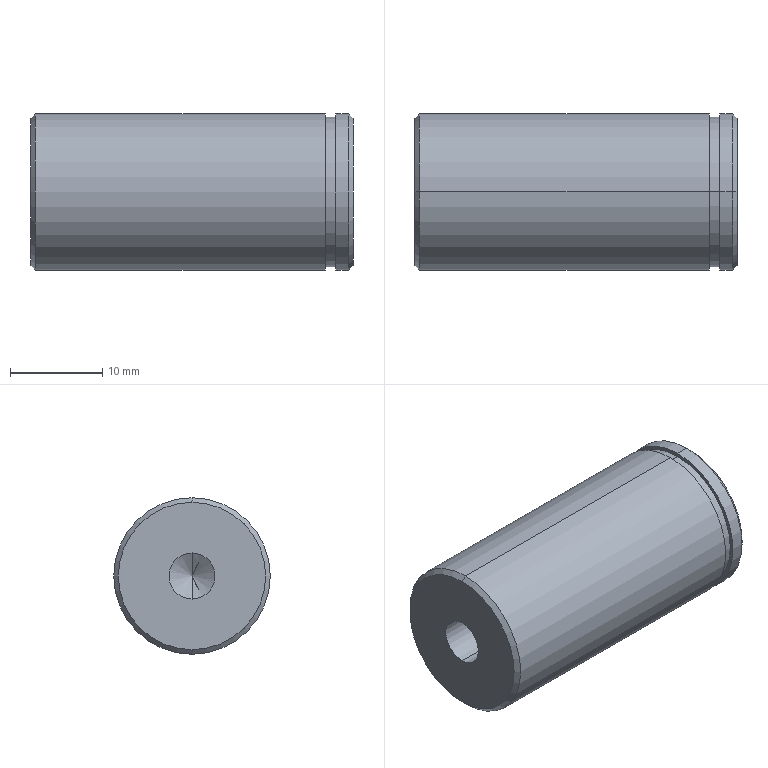Part | SolidWorks | features Chamfer 1, Extrusion 1, HoleWzd 1, RevCut 1 | 1 solid | 18 faces | box 35 x 17 x 17 mm | volume 7604 mm3 | cylinder 8 | cone 6 | plane 4 | commonest cylinder face diameters 17 x4 5 x2 16.2 x2
STEP:
#1=CARTESIAN_POINT('',(34.5,0.,8.5));
#2=VERTEX_POINT('',#1);
#3=CARTESIAN_POINT('',(34.5,0.,-8.5));
#4=VERTEX_POINT('',#3);
#5=CARTESIAN_POINT('',(34.5,0.,0.));
#6=DIRECTION('',(-1.,0.,0.));
#7=DIRECTION('',(0.,0.,-1.));
#8=AXIS2_PLACEMENT_3D('',#5,#6,#7);
#9=CIRCLE('',#8,8.5);
#10=EDGE_CURVE('',#2,#4,#9,.T.);
#11=ORIENTED_EDGE('',*,*,#10,.T.);
#12=CARTESIAN_POINT('',(33.1,0.,-8.5));
#13=VERTEX_POINT('',#12);
#14=CARTESIAN_POINT('',(35.,0.,-8.5));
#15=DIRECTION('',(-1.,0.,0.));
#16=VECTOR('',#15,1000.);
#17=LINE('',#14,#16);
#18=EDGE_CURVE('',#4,#13,#17,.T.);
#19=ORIENTED_EDGE('',*,*,#18,.T.);
#20=CARTESIAN_POINT('',(33.1,0.,8.5));
#21=VERTEX_POINT('',#20);
#22=CARTESIAN_POINT('',(33.1,0.,0.));
#23=DIRECTION('',(-1.,0.,0.));
#24=DIRECTION('',(0.,0.,1.));
#25=AXIS2_PLACEMENT_3D('',#22,#23,#24);
#26=CIRCLE('',#25,8.5);
#27=EDGE_CURVE('',#21,#13,#26,.T.);
#28=ORIENTED_EDGE('',*,*,#27,.F.);
#29=CARTESIAN_POINT('',(35.,0.,8.5));
#30=DIRECTION('',(-1.,0.,0.));
#31=VECTOR('',#30,1000.);
#32=LINE('',#29,#31);
#33=EDGE_CURVE('',#2,#21,#32,.T.);
#34=ORIENTED_EDGE('',*,*,#33,.F.);
#35=EDGE_LOOP('',(#11,#19,#28,#34));
#36=FACE_OUTER_BOUND('',#35,.T.);
#37=CARTESIAN_POINT('',(35.,0.,0.));
#38=DIRECTION('',(-1.,0.,0.));
#39=DIRECTION('',(0.,0.,1.));
#40=AXIS2_PLACEMENT_3D('',#37,#38,#39);
#41=CYLINDRICAL_SURFACE('',#40,8.5);
#42=ADVANCED_FACE('',(#36),#41,.T.);
#43=CARTESIAN_POINT('',(35.,0.,-8.));
#44=VERTEX_POINT('',#43);
#45=CARTESIAN_POINT('',(35.,0.,8.));
#46=VERTEX_POINT('',#45);
#47=CARTESIAN_POINT('',(35.,0.,0.));
#48=DIRECTION('',(1.,0.,0.));
#49=DIRECTION('',(0.,0.,-1.));
#50=AXIS2_PLACEMENT_3D('',#47,#48,#49);
#51=CIRCLE('',#50,8.);
#52=EDGE_CURVE('',#44,#46,#51,.T.);
#53=ORIENTED_EDGE('',*,*,#52,.F.);
#54=CARTESIAN_POINT('',(35.,0.,-8.));
#55=DIRECTION('',(-0.7071,0.,-0.7071));
#56=VECTOR('',#55,1000.);
#57=LINE('',#54,#56);
#58=EDGE_CURVE('',#44,#4,#57,.T.);
#59=ORIENTED_EDGE('',*,*,#58,.T.);
#60=ORIENTED_EDGE('',*,*,#10,.F.);
#61=CARTESIAN_POINT('',(35.,0.,8.));
#62=DIRECTION('',(-0.7071,0.,0.7071));
#63=VECTOR('',#62,1000.);
#64=LINE('',#61,#63);
#65=EDGE_CURVE('',#46,#2,#64,.T.);
#66=ORIENTED_EDGE('',*,*,#65,.F.);
#67=EDGE_LOOP('',(#53,#59,#60,#66));
#68=FACE_OUTER_BOUND('',#67,.T.);
#69=CARTESIAN_POINT('',(35.,0.,0.));
#70=DIRECTION('',(-1.,0.,0.));
#71=DIRECTION('',(0.,0.,1.));
#72=AXIS2_PLACEMENT_3D('',#69,#70,#71);
#73=CONICAL_SURFACE('',#72,8.,0.7854);
#74=ADVANCED_FACE('',(#68),#73,.T.);
#75=CARTESIAN_POINT('',(33.1,0.,8.1));
#76=VERTEX_POINT('',#75);
#77=CARTESIAN_POINT('',(33.1,0.,-8.1));
#78=VERTEX_POINT('',#77);
#79=CARTESIAN_POINT('',(33.1,0.,0.));
#80=DIRECTION('',(-1.,0.,0.));
#81=DIRECTION('',(0.,0.,1.));
#82=AXIS2_PLACEMENT_3D('',#79,#80,#81);
#83=CIRCLE('',#82,8.1);
#84=EDGE_CURVE('',#76,#78,#83,.T.);
#85=ORIENTED_EDGE('',*,*,#84,.T.);
#86=CARTESIAN_POINT('',(32.,0.,-8.1));
#87=VERTEX_POINT('',#86);
#88=CARTESIAN_POINT('',(-5.278,0.,-8.1));
#89=DIRECTION('',(-1.,0.,0.));
#90=VECTOR('',#89,1000.);
#91=LINE('',#88,#90);
#92=EDGE_CURVE('',#78,#87,#91,.T.);
#93=ORIENTED_EDGE('',*,*,#92,.T.);
#94=CARTESIAN_POINT('',(32.,0.,8.1));
#95=VERTEX_POINT('',#94);
#96=CARTESIAN_POINT('',(32.,0.,0.));
#97=DIRECTION('',(-1.,0.,0.));
#98=DIRECTION('',(0.,0.,1.));
#99=AXIS2_PLACEMENT_3D('',#96,#97,#98);
#100=CIRCLE('',#99,8.1);
#101=EDGE_CURVE('',#95,#87,#100,.T.);
#102=ORIENTED_EDGE('',*,*,#101,.F.);
#103=CARTESIAN_POINT('',(-5.278,0.,8.1));
#104=DIRECTION('',(-1.,0.,0.));
#105=VECTOR('',#104,1000.);
#106=LINE('',#103,#105);
#107=EDGE_CURVE('',#76,#95,#106,.T.);
#108=ORIENTED_EDGE('',*,*,#107,.F.);
#109=EDGE_LOOP('',(#85,#93,#102,#108));
#110=FACE_OUTER_BOUND('',#109,.T.);
#111=CARTESIAN_POINT('',(-5.278,0.,0.));
#112=DIRECTION('',(-1.,0.,0.));
#113=DIRECTION('',(0.,0.,1.));
#114=AXIS2_PLACEMENT_3D('',#111,#112,#113);
#115=CYLINDRICAL_SURFACE('',#114,8.1);
#116=ADVANCED_FACE('',(#110),#115,.T.);
#117=CARTESIAN_POINT('',(0.,0.,8.));
#118=VERTEX_POINT('',#117);
#119=CARTESIAN_POINT('',(0.,0.,-8.));
#120=VERTEX_POINT('',#119);
#121=CARTESIAN_POINT('',(0.,0.,0.));
#122=DIRECTION('',(-1.,0.,0.));
#123=DIRECTION('',(0.,0.,-1.));
#124=AXIS2_PLACEMENT_3D('',#121,#122,#123);
#125=CIRCLE('',#124,8.);
#126=EDGE_CURVE('',#118,#120,#125,.T.);
#127=ORIENTED_EDGE('',*,*,#126,.F.);
#128=CARTESIAN_POINT('',(0.5,0.,8.5));
#129=VERTEX_POINT('',#128);
#130=CARTESIAN_POINT('',(0.5,0.,8.5));
#131=DIRECTION('',(0.7071,0.,0.7071));
#132=VECTOR('',#131,1000.);
#133=LINE('',#130,#132);
#134=EDGE_CURVE('',#118,#129,#133,.T.);
#135=ORIENTED_EDGE('',*,*,#134,.T.);
#136=CARTESIAN_POINT('',(0.5,0.,-8.5));
#137=VERTEX_POINT('',#136);
#138=CARTESIAN_POINT('',(0.5,0.,0.));
#139=DIRECTION('',(1.,0.,0.));
#140=DIRECTION('',(0.,0.,-1.));
#141=AXIS2_PLACEMENT_3D('',#138,#139,#140);
#142=CIRCLE('',#141,8.5);
#143=EDGE_CURVE('',#137,#129,#142,.T.);
#144=ORIENTED_EDGE('',*,*,#143,.F.);
#145=CARTESIAN_POINT('',(0.5,0.,-8.5));
#146=DIRECTION('',(0.7071,0.,-0.7071));
#147=VECTOR('',#146,1000.);
#148=LINE('',#145,#147);
#149=EDGE_CURVE('',#120,#137,#148,.T.);
#150=ORIENTED_EDGE('',*,*,#149,.F.);
#151=EDGE_LOOP('',(#127,#135,#144,#150));
#152=FACE_OUTER_BOUND('',#151,.T.);
#153=CARTESIAN_POINT('',(0.5,0.,0.));
#154=DIRECTION('',(1.,0.,0.));
#155=DIRECTION('',(0.,0.,-1.));
#156=AXIS2_PLACEMENT_3D('',#153,#154,#155);
#157=CONICAL_SURFACE('',#156,8.5,0.7854);
#158=ADVANCED_FACE('',(#152),#157,.T.);
#159=CARTESIAN_POINT('',(15.,0.,-2.5));
#160=VERTEX_POINT('',#159);
#161=CARTESIAN_POINT('',(15.,0.,2.5));
#162=VERTEX_POINT('',#161);
#163=CARTESIAN_POINT('',(15.,0.,0.));
#164=DIRECTION('',(-1.,0.,0.));
#165=DIRECTION('',(0.,0.,1.));
#166=AXIS2_PLACEMENT_3D('',#163,#164,#165);
#167=CIRCLE('',#166,2.5);
#168=EDGE_CURVE('',#160,#162,#167,.T.);
#169=ORIENTED_EDGE('',*,*,#168,.F.);
#170=CARTESIAN_POINT('',(0.,0.,-2.5));
#171=VERTEX_POINT('',#170);
#172=CARTESIAN_POINT('',(0.,0.,-2.5));
#173=DIRECTION('',(-1.,0.,0.));
#174=VECTOR('',#173,1000.);
#175=LINE('',#172,#174);
#176=EDGE_CURVE('',#160,#171,#175,.T.);
#177=ORIENTED_EDGE('',*,*,#176,.T.);
#178=CARTESIAN_POINT('',(0.,0.,2.5));
#179=VERTEX_POINT('',#178);
#180=CARTESIAN_POINT('',(0.,0.,0.));
#181=DIRECTION('',(-1.,0.,0.));
#182=DIRECTION('',(0.,0.,1.));
#183=AXIS2_PLACEMENT_3D('',#180,#181,#182);
#184=CIRCLE('',#183,2.5);
#185=EDGE_CURVE('',#171,#179,#184,.T.);
#186=ORIENTED_EDGE('',*,*,#185,.T.);
#187=CARTESIAN_POINT('',(0.,0.,2.5));
#188=DIRECTION('',(-1.,0.,0.));
#189=VECTOR('',#188,1000.);
#190=LINE('',#187,#189);
#191=EDGE_CURVE('',#162,#179,#190,.T.);
#192=ORIENTED_EDGE('',*,*,#191,.F.);
#193=EDGE_LOOP('',(#169,#177,#186,#192));
#194=FACE_OUTER_BOUND('',#193,.T.);
#195=CARTESIAN_POINT('',(0.,0.,0.));
#196=DIRECTION('',(-1.,0.,0.));
#197=DIRECTION('',(0.,0.,1.));
#198=AXIS2_PLACEMENT_3D('',#195,#196,#197);
#199=CYLINDRICAL_SURFACE('',#198,2.5);
#200=ADVANCED_FACE('',(#194),#199,.F.);
#201=CARTESIAN_POINT('',(16.502,0.,0.));
#202=VERTEX_POINT('',#201);
#203=CARTESIAN_POINT('',(15.,0.,2.5));
#204=DIRECTION('',(-0.515,0.,0.8572));
#205=VECTOR('',#204,1000.);
#206=LINE('',#203,#205);
#207=EDGE_CURVE('',#202,#162,#206,.T.);
#208=ORIENTED_EDGE('',*,*,#207,.F.);
#209=CARTESIAN_POINT('',(15.,0.,-2.5));
#210=DIRECTION('',(-0.515,0.,-0.8572));
#211=VECTOR('',#210,1000.);
#212=LINE('',#209,#211);
#213=EDGE_CURVE('',#202,#160,#212,.T.);
#214=ORIENTED_EDGE('',*,*,#213,.T.);
#215=ORIENTED_EDGE('',*,*,#168,.T.);
#216=EDGE_LOOP('',(#208,#214,#215));
#217=FACE_OUTER_BOUND('',#216,.T.);
#218=CARTESIAN_POINT('',(15.,0.,0.));
#219=DIRECTION('',(-1.,0.,0.));
#220=DIRECTION('',(0.,0.,1.));
#221=AXIS2_PLACEMENT_3D('',#218,#219,#220);
#222=CONICAL_SURFACE('',#221,2.5,1.03);
#223=ADVANCED_FACE('',(#217),#222,.F.);
#224=CARTESIAN_POINT('',(32.,0.,-8.5));
#225=VERTEX_POINT('',#224);
#226=CARTESIAN_POINT('',(32.,0.,8.5));
#227=VERTEX_POINT('',#226);
#228=CARTESIAN_POINT('',(32.,0.,0.));
#229=DIRECTION('',(1.,0.,0.));
#230=DIRECTION('',(0.,0.,-1.));
#231=AXIS2_PLACEMENT_3D('',#228,#229,#230);
#232=CIRCLE('',#231,8.5);
#233=EDGE_CURVE('',#225,#227,#232,.T.);
#234=ORIENTED_EDGE('',*,*,#233,.F.);
#235=CARTESIAN_POINT('',(35.,0.,-8.5));
#236=DIRECTION('',(-1.,0.,0.));
#237=VECTOR('',#236,1000.);
#238=LINE('',#235,#237);
#239=EDGE_CURVE('',#225,#137,#238,.T.);
#240=ORIENTED_EDGE('',*,*,#239,.T.);
#241=ORIENTED_EDGE('',*,*,#143,.T.);
#242=CARTESIAN_POINT('',(35.,0.,8.5));
#243=DIRECTION('',(-1.,0.,0.));
#244=VECTOR('',#243,1000.);
#245=LINE('',#242,#244);
#246=EDGE_CURVE('',#227,#129,#245,.T.);
#247=ORIENTED_EDGE('',*,*,#246,.F.);
#248=EDGE_LOOP('',(#234,#240,#241,#247));
#249=FACE_OUTER_BOUND('',#248,.T.);
#250=CARTESIAN_POINT('',(35.,0.,0.));
#251=DIRECTION('',(-1.,0.,0.));
#252=DIRECTION('',(0.,0.,1.));
#253=AXIS2_PLACEMENT_3D('',#250,#251,#252);
#254=CYLINDRICAL_SURFACE('',#253,8.5);
#255=ADVANCED_FACE('',(#249),#254,.T.);
#256=ORIENTED_EDGE('',*,*,#239,.F.);
#257=CARTESIAN_POINT('',(32.,0.,0.));
#258=DIRECTION('',(1.,0.,0.));
#259=DIRECTION('',(0.,0.,-1.));
#260=AXIS2_PLACEMENT_3D('',#257,#258,#259);
#261=CIRCLE('',#260,8.5);
#262=EDGE_CURVE('',#227,#225,#261,.T.);
#263=ORIENTED_EDGE('',*,*,#262,.F.);
#264=ORIENTED_EDGE('',*,*,#246,.T.);
#265=CARTESIAN_POINT('',(0.5,0.,0.));
#266=DIRECTION('',(1.,0.,0.));
#267=DIRECTION('',(0.,0.,-1.));
#268=AXIS2_PLACEMENT_3D('',#265,#266,#267);
#269=CIRCLE('',#268,8.5);
#270=EDGE_CURVE('',#129,#137,#269,.T.);
#271=ORIENTED_EDGE('',*,*,#270,.T.);
#272=EDGE_LOOP('',(#256,#263,#264,#271));
#273=FACE_OUTER_BOUND('',#272,.T.);
#274=CARTESIAN_POINT('',(35.,0.,0.));
#275=DIRECTION('',(-1.,0.,0.));
#276=DIRECTION('',(0.,0.,1.));
#277=AXIS2_PLACEMENT_3D('',#274,#275,#276);
#278=CYLINDRICAL_SURFACE('',#277,8.5);
#279=ADVANCED_FACE('',(#273),#278,.T.);
#280=CARTESIAN_POINT('',(0.,0.,0.));
#281=DIRECTION('',(-1.,0.,0.));
#282=DIRECTION('',(0.,0.,-1.));
#283=AXIS2_PLACEMENT_3D('',#280,#281,#282);
#284=CIRCLE('',#283,8.);
#285=EDGE_CURVE('',#120,#118,#284,.T.);
#286=ORIENTED_EDGE('',*,*,#285,.T.);
#287=ORIENTED_EDGE('',*,*,#126,.T.);
#288=EDGE_LOOP('',(#286,#287));
#289=FACE_OUTER_BOUND('',#288,.T.);
#290=CARTESIAN_POINT('',(0.,0.,0.));
#291=DIRECTION('',(-1.,0.,0.));
#292=DIRECTION('',(0.,0.,1.));
#293=AXIS2_PLACEMENT_3D('',#290,#291,#292);
#294=CIRCLE('',#293,2.5);
#295=EDGE_CURVE('',#179,#171,#294,.T.);
#296=ORIENTED_EDGE('',*,*,#295,.F.);
#297=ORIENTED_EDGE('',*,*,#185,.F.);
#298=EDGE_LOOP('',(#296,#297));
#299=FACE_BOUND('',#298,.T.);
#300=CARTESIAN_POINT('',(0.,0.,0.));
#301=DIRECTION('',(1.,0.,0.));
#302=DIRECTION('',(0.,0.,-1.));
#303=AXIS2_PLACEMENT_3D('',#300,#301,#302);
#304=PLANE('',#303);
#305=ADVANCED_FACE('',(#289,#299),#304,.F.);
#306=ORIENTED_EDGE('',*,*,#213,.F.);
#307=ORIENTED_EDGE('',*,*,#207,.T.);
#308=CARTESIAN_POINT('',(15.,0.,0.));
#309=DIRECTION('',(-1.,0.,0.));
#310=DIRECTION('',(0.,0.,1.));
#311=AXIS2_PLACEMENT_3D('',#308,#309,#310);
#312=CIRCLE('',#311,2.5);
#313=EDGE_CURVE('',#162,#160,#312,.T.);
#314=ORIENTED_EDGE('',*,*,#313,.T.);
#315=EDGE_LOOP('',(#306,#307,#314));
#316=FACE_OUTER_BOUND('',#315,.T.);
#317=CARTESIAN_POINT('',(15.,0.,0.));
#318=DIRECTION('',(-1.,0.,0.));
#319=DIRECTION('',(0.,0.,1.));
#320=AXIS2_PLACEMENT_3D('',#317,#318,#319);
#321=CONICAL_SURFACE('',#320,2.5,1.03);
#322=ADVANCED_FACE('',(#316),#321,.F.);
#323=ORIENTED_EDGE('',*,*,#176,.F.);
#324=ORIENTED_EDGE('',*,*,#313,.F.);
#325=ORIENTED_EDGE('',*,*,#191,.T.);
#326=ORIENTED_EDGE('',*,*,#295,.T.);
#327=EDGE_LOOP('',(#323,#324,#325,#326));
#328=FACE_OUTER_BOUND('',#327,.T.);
#329=CARTESIAN_POINT('',(0.,0.,0.));
#330=DIRECTION('',(-1.,0.,0.));
#331=DIRECTION('',(0.,0.,1.));
#332=AXIS2_PLACEMENT_3D('',#329,#330,#331);
#333=CYLINDRICAL_SURFACE('',#332,2.5);
#334=ADVANCED_FACE('',(#328),#333,.F.);
#335=ORIENTED_EDGE('',*,*,#134,.F.);
#336=ORIENTED_EDGE('',*,*,#285,.F.);
#337=ORIENTED_EDGE('',*,*,#149,.T.);
#338=ORIENTED_EDGE('',*,*,#270,.F.);
#339=EDGE_LOOP('',(#335,#336,#337,#338));
#340=FACE_OUTER_BOUND('',#339,.T.);
#341=CARTESIAN_POINT('',(0.5,0.,0.));
#342=DIRECTION('',(1.,0.,0.));
#343=DIRECTION('',(0.,0.,-1.));
#344=AXIS2_PLACEMENT_3D('',#341,#342,#343);
#345=CONICAL_SURFACE('',#344,8.5,0.7854);
#346=ADVANCED_FACE('',(#340),#345,.T.);
#347=ORIENTED_EDGE('',*,*,#101,.T.);
#348=CARTESIAN_POINT('',(32.,0.,0.));
#349=DIRECTION('',(-1.,0.,0.));
#350=DIRECTION('',(0.,0.,1.));
#351=AXIS2_PLACEMENT_3D('',#348,#349,#350);
#352=CIRCLE('',#351,8.1);
#353=EDGE_CURVE('',#87,#95,#352,.T.);
#354=ORIENTED_EDGE('',*,*,#353,.T.);
#355=EDGE_LOOP('',(#347,#354));
#356=FACE_BOUND('',#355,.T.);
#357=ORIENTED_EDGE('',*,*,#262,.T.);
#358=ORIENTED_EDGE('',*,*,#233,.T.);
#359=EDGE_LOOP('',(#357,#358));
#360=FACE_OUTER_BOUND('',#359,.T.);
#361=CARTESIAN_POINT('',(32.,0.,-10.865));
#362=DIRECTION('',(1.,0.,0.));
#363=DIRECTION('',(0.,0.,-1.));
#364=AXIS2_PLACEMENT_3D('',#361,#362,#363);
#365=PLANE('',#364);
#366=ADVANCED_FACE('',(#356,#360),#365,.T.);
#367=ORIENTED_EDGE('',*,*,#84,.F.);
#368=CARTESIAN_POINT('',(33.1,0.,0.));
#369=DIRECTION('',(-1.,0.,0.));
#370=DIRECTION('',(0.,0.,1.));
#371=AXIS2_PLACEMENT_3D('',#368,#369,#370);
#372=CIRCLE('',#371,8.1);
#373=EDGE_CURVE('',#78,#76,#372,.T.);
#374=ORIENTED_EDGE('',*,*,#373,.F.);
#375=EDGE_LOOP('',(#367,#374));
#376=FACE_BOUND('',#375,.T.);
#377=ORIENTED_EDGE('',*,*,#27,.T.);
#378=CARTESIAN_POINT('',(33.1,0.,0.));
#379=DIRECTION('',(-1.,0.,0.));
#380=DIRECTION('',(0.,0.,1.));
#381=AXIS2_PLACEMENT_3D('',#378,#379,#380);
#382=CIRCLE('',#381,8.5);
#383=EDGE_CURVE('',#13,#21,#382,.T.);
#384=ORIENTED_EDGE('',*,*,#383,.T.);
#385=EDGE_LOOP('',(#377,#384));
#386=FACE_OUTER_BOUND('',#385,.T.);
#387=CARTESIAN_POINT('',(33.1,0.,-10.865));
#388=DIRECTION('',(-1.,0.,0.));
#389=DIRECTION('',(0.,0.,1.));
#390=AXIS2_PLACEMENT_3D('',#387,#388,#389);
#391=PLANE('',#390);
#392=ADVANCED_FACE('',(#376,#386),#391,.T.);
#393=ORIENTED_EDGE('',*,*,#92,.F.);
#394=ORIENTED_EDGE('',*,*,#373,.T.);
#395=ORIENTED_EDGE('',*,*,#107,.T.);
#396=ORIENTED_EDGE('',*,*,#353,.F.);
#397=EDGE_LOOP('',(#393,#394,#395,#396));
#398=FACE_OUTER_BOUND('',#397,.T.);
#399=CARTESIAN_POINT('',(-5.278,0.,0.));
#400=DIRECTION('',(-1.,0.,0.));
#401=DIRECTION('',(0.,0.,1.));
#402=AXIS2_PLACEMENT_3D('',#399,#400,#401);
#403=CYLINDRICAL_SURFACE('',#402,8.1);
#404=ADVANCED_FACE('',(#398),#403,.T.);
#405=CARTESIAN_POINT('',(35.,0.,0.));
#406=DIRECTION('',(1.,0.,0.));
#407=DIRECTION('',(0.,0.,-1.));
#408=AXIS2_PLACEMENT_3D('',#405,#406,#407);
#409=CIRCLE('',#408,8.);
#410=EDGE_CURVE('',#46,#44,#409,.T.);
#411=ORIENTED_EDGE('',*,*,#410,.T.);
#412=ORIENTED_EDGE('',*,*,#52,.T.);
#413=EDGE_LOOP('',(#411,#412));
#414=FACE_OUTER_BOUND('',#413,.T.);
#415=CARTESIAN_POINT('',(35.,0.,0.));
#416=DIRECTION('',(1.,0.,0.));
#417=DIRECTION('',(0.,0.,-1.));
#418=AXIS2_PLACEMENT_3D('',#415,#416,#417);
#419=PLANE('',#418);
#420=ADVANCED_FACE('',(#414),#419,.T.);
#421=ORIENTED_EDGE('',*,*,#58,.F.);
#422=ORIENTED_EDGE('',*,*,#410,.F.);
#423=ORIENTED_EDGE('',*,*,#65,.T.);
#424=CARTESIAN_POINT('',(34.5,0.,0.));
#425=DIRECTION('',(-1.,0.,0.));
#426=DIRECTION('',(0.,0.,-1.));
#427=AXIS2_PLACEMENT_3D('',#424,#425,#426);
#428=CIRCLE('',#427,8.5);
#429=EDGE_CURVE('',#4,#2,#428,.T.);
#430=ORIENTED_EDGE('',*,*,#429,.F.);
#431=EDGE_LOOP('',(#421,#422,#423,#430));
#432=FACE_OUTER_BOUND('',#431,.T.);
#433=CARTESIAN_POINT('',(35.,0.,0.));
#434=DIRECTION('',(-1.,0.,0.));
#435=DIRECTION('',(0.,0.,1.));
#436=AXIS2_PLACEMENT_3D('',#433,#434,#435);
#437=CONICAL_SURFACE('',#436,8.,0.7854);
#438=ADVANCED_FACE('',(#432),#437,.T.);
#439=ORIENTED_EDGE('',*,*,#18,.F.);
#440=ORIENTED_EDGE('',*,*,#429,.T.);
#441=ORIENTED_EDGE('',*,*,#33,.T.);
#442=ORIENTED_EDGE('',*,*,#383,.F.);
#443=EDGE_LOOP('',(#439,#440,#441,#442));
#444=FACE_OUTER_BOUND('',#443,.T.);
#445=CARTESIAN_POINT('',(35.,0.,0.));
#446=DIRECTION('',(-1.,0.,0.));
#447=DIRECTION('',(0.,0.,1.));
#448=AXIS2_PLACEMENT_3D('',#445,#446,#447);
#449=CYLINDRICAL_SURFACE('',#448,8.5);
#450=ADVANCED_FACE('',(#444),#449,.T.);
#451=CLOSED_SHELL('',(#42,#74,#116,#158,#200,#223,#255,#279,#305,#322,#334,#346,#366,#392,#404,#420,#438,#450));
#452=MANIFOLD_SOLID_BREP('',#451);
#453=CARTESIAN_POINT('',(0.,0.,0.));
#454=DIRECTION('',(0.,0.,1.));
#455=DIRECTION('',(1.,0.,0.));
#456=AXIS2_PLACEMENT_3D('',#453,#454,#455);
#457=(LENGTH_UNIT()NAMED_UNIT(*)SI_UNIT(.MILLI.,.METRE.));
#458=UNCERTAINTY_MEASURE_WITH_UNIT(LENGTH_MEASURE(0.00001),#457,'','');
#459=(NAMED_UNIT(*)PLANE_ANGLE_UNIT()SI_UNIT($,.RADIAN.));
#460=(NAMED_UNIT(*)SI_UNIT($,.STERADIAN.)SOLID_ANGLE_UNIT());
#461=(GEOMETRIC_REPRESENTATION_CONTEXT(3)GLOBAL_UNCERTAINTY_ASSIGNED_CONTEXT((#458))GLOBAL_UNIT_ASSIGNED_CONTEXT((#457,#459,#460))REPRESENTATION_CONTEXT('',''));
#462=ADVANCED_BREP_SHAPE_REPRESENTATION('',(#452,#456),#461);